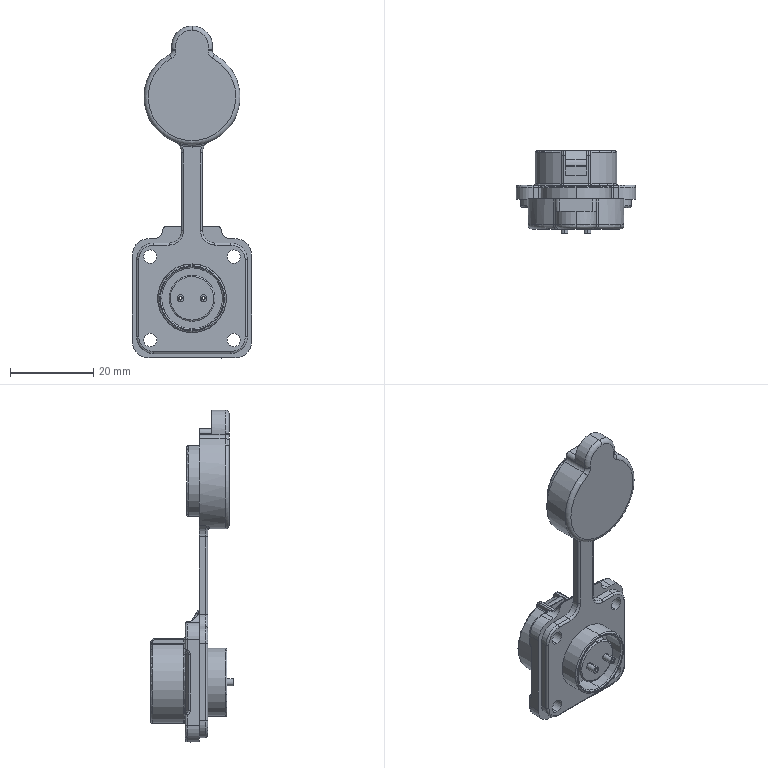Part | SolidWorks | features BaseBody 1 | 1 solid | 257 faces | box 28.601 x 19.7 x 79.542 mm | volume 7374 mm3 | cylinder 120 | plane 56 | torus 51 | spline 17 | cone 8 | sphere 5 | commonest cylinder face diameters 1 x24 2 x10 0.6 x9 1.6 x8 3.2 x8 5.8 x8